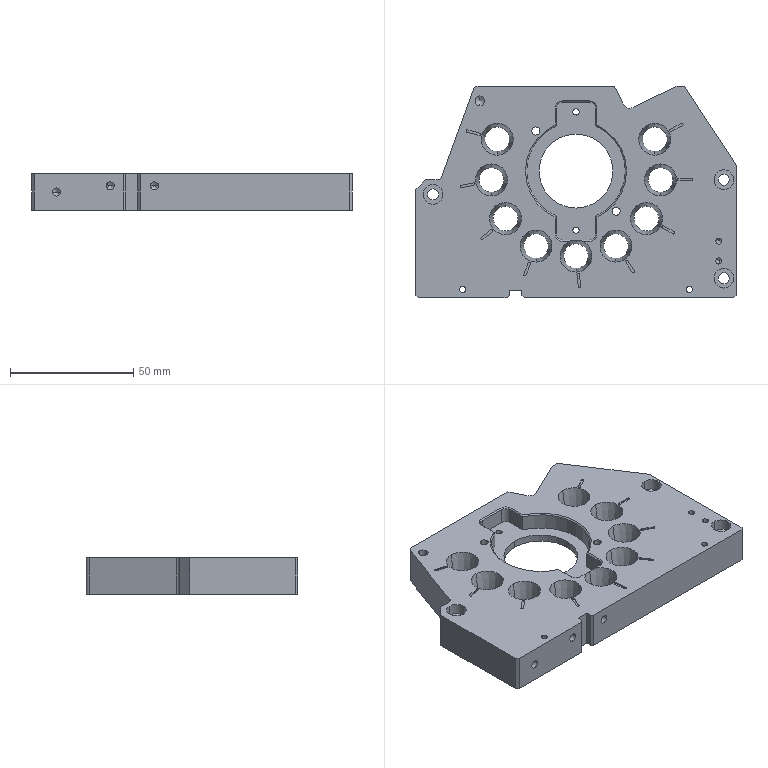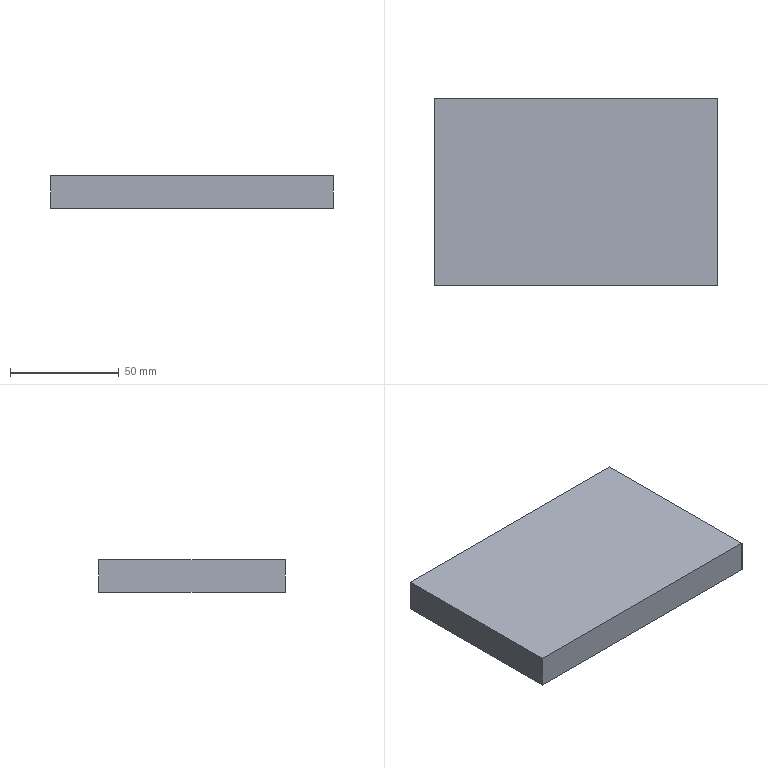CAM job | NX | 3+2 milling, drilling | part box 130 x 86 x 15 mm | stock box 130 x 86 x 15 mm
Tools:
number,name,description,diameter,corner_radius,flute_length,length,flutes
21,ZXZ,Milling Tool-5 Parameters,6.0,0.0,50.0,75.0,2
22,2.5ZT,Drilling Tool,2.5,0.0,35.0,50.0,2
13,3.3ZT,Drilling Tool,3.3,0.0,35.0,50.0,2
24,4.0ZT,Drilling Tool,4.0,0.0,35.0,50.0,2
12,4.5ZT,Drilling Tool,4.5,0.0,35.0,50.0,2
4,D10,Milling Tool-5 Parameters,10.0,0.0,50.0,75.0,2
20,10.ZT,Drilling Tool,10.0,0.0,35.0,50.0,2
17,D4,Milling Tool-5 Parameters,4.0,0.0,50.0,75.0,2
6,D6,Milling Tool-5 Parameters,6.0,0.0,50.0,75.0,2
16,D6JING,Milling Tool-5 Parameters,6.0,0.0,50.0,75.0,2
7,D4R0.5,Milling Tool-5 Parameters,4.0,0.5,50.0,75.0,2
19,D1,Milling Tool-5 Parameters,1.0,0.0,50.0,75.0,2
1,D6A45,Milling Tool-5 Parameters,6.0,0.0,50.0,75.0,2
Operations:
program,operation,operation_type,tool,method,geometry_group,spindle_rpm,surface_speed,feed_per_tooth,feed_cut,feed_plunge,cut_length_mm,path_length_mm,cut_time_min,machine_time_min
1,DRILLING,Operation,ZXZ,METHOD,A,3500.0,65.0,0.0357,250.0,0.0,84.0,690.801,0.336,0.3967
1,DRILLING_COPY_COPY,Operation,2.5ZT,METHOD,A,2000.0,21.0,0.0375,150.0,0.0,103.507,485.801,0.69,0.7283
1,DRILLING_COPY_1,Operation,3.3ZT,METHOD,A,2000.0,21.0,0.0375,150.0,0.0,30.983,171.063,0.2066,0.2206
1,DRILLING_COPY_1_COPY,Operation,4.0ZT,METHOD,A,2000.0,21.0,0.0375,150.0,0.0,9.202,78.403,0.0613,0.0683
1,DRILLING_COPY,Operation,4.5ZT,METHOD,A,2000.0,28.0,0.0375,150.0,0.0,62.556,349.414,0.417,0.4457
1,DRILLING_COPY_COPY_1,Operation,10.ZT,METHOD,A,2000.0,28.0,0.0375,150.0,0.0,202.539,624.758,1.35,1.393
1,ZLEVEL_PROFILE,ZLevelMilling,D10,METHOD,A,3500.0,109.0,0.3143,2200.0,1000.0,9960.656,10284.389,4.731,4.763
1,ADAPTIVE_MILLING,CavityMilling,D10,METHOD,A,7500.0,235.0,0.2,3000.0,1000.0,11162.735,11585.71,5.695,5.738
1,HOLE_MILLING_COPY,CylinderMilling,D6,METHOD,A,5500.0,103.0,0.1364,1500.0,100.0,989.723,1340.176,0.6598,0.6949
1,FLOOR_WALL_1_COPY,VolumeBased25DMillingOperation,D6JING,METHOD,A,7500.0,235.0,0.08,1200.0,1000.0,568.072,639.972,0.4743,0.4815
1,ZLEVEL_PROFILE_2,ZLevelMilling,D6JING,METHOD,A,7500.0,235.0,0.0667,1000.0,100.0,152.755,468.87,0.1528,0.1844
1,ZLEVEL_PROFILE_2_COPY,ZLevelMilling,D6JING,METHOD,A,7500.0,235.0,0.0667,1000.0,100.0,68.474,241.468,0.0685,0.0858
1,ZLEVEL_PROFILE_1,ZLevelMilling,D4,METHOD,A,6500.0,81.0,0.1269,1650.0,100.0,2028.876,3364.187,1.23,1.363
1,ZLEVEL_PROFILE_1_COPY,ZLevelMilling,D4,METHOD,A,6500.0,81.0,0.1269,1650.0,100.0,2070.891,3417.953,1.255,1.39
1,ZLEVEL_PROFILE_1_1,ZLevelMilling,D4R0.5,METHOD,A,7500.0,94.0,0.1667,2500.0,1000.0,22890.897,23935.847,9.168,9.273
1,PLANAR_PROFILE,PlanarMilling,D1,METHOD,A,6500.0,20.0,0.0615,800.0,100.0,4954.5,5607.402,6.193,6.258
1,PLANAR_MILL,PlanarMilling,D6A45,METHOD,A,7500.0,141.0,0.0833,1250.0,100.0,531.11,1965.382,0.4249,0.5683
1,PLANAR_MILL_COPY_1,PlanarMilling,D6A45,METHOD,A,7500.0,141.0,0.0833,1250.0,100.0,96.783,168.783,0.0774,0.0846
1,PLANAR_MILL_COPY,PlanarMilling,D6A45,METHOD,A,7500.0,141.0,0.0833,1250.0,100.0,158.298,217.298,0.1266,0.1325
1,刀补16,ZLevelMilling,D6JING,METHOD,A,7500.0,235.0,0.0667,1000.0,100.0,101.807,250.637,0.1018,0.1167
1,刀补16_COPY,ZLevelMilling,D4,METHOD,A,7500.0,235.0,0.0667,1000.0,100.0,86.152,164.152,0.0862,0.094
2,ADAPTIVE_MILLING_COPY,CavityMilling,D10,METHOD,B,7500.0,235.0,0.2,3000.0,1000.0,11734.765,12049.371,4.22,4.251
2,FLOOR_WALL_1_COPY_COPY,VolumeBased25DMillingOperation,D6JING,METHOD,B,7500.0,235.0,0.08,1200.0,1000.0,702.647,770.547,0.5864,0.5932
2,ZLEVEL_PROFILE_1_COPY_COPY,ZLevelMilling,D4,METHOD,B,6500.0,81.0,0.1269,1650.0,100.0,1560.563,2689.973,0.9458,1.059
2,PLANAR_MILL_COPY_1_COPY,PlanarMilling,D6A45,METHOD,B,7500.0,141.0,0.0833,1250.0,100.0,96.783,164.783,0.0774,0.0842
2,PLANAR_MILL_COPY_1_COPY_COPY,PlanarMilling,D6A45,METHOD,B,7500.0,141.0,0.0833,1250.0,100.0,568.881,1935.207,0.4551,0.5917
3,DRILLING_COPY_2,Operation,ZXZ,METHOD,C,3500.0,65.0,0.0357,250.0,0.0,12.0,152.039,0.048,0.062
3,DRILLING_COPY_1_COPY_1,Operation,3.3ZT,METHOD,C,2000.0,21.0,0.0375,150.0,0.0,37.174,202.388,0.2478,0.2643
3,ZLEVEL_PROFILE_1_COPY_COPY_1,ZLevelMilling,D4,METHOD,C,7500.0,141.0,0.11,1650.0,1000.0,1450.778,1512.678,0.8802,0.8864
3,PLANAR_MILL_COPY_1_COPY_COPY_1,PlanarMilling,D6A45,METHOD,C,7500.0,141.0,0.0833,1250.0,100.0,45.891,166.491,0.0367,0.0488
3,PLANAR_MILL_COPY_1_COPY_COPY_1_COPY,PlanarMilling,D6A45,METHOD,C,7500.0,141.0,0.0833,1250.0,100.0,48.398,264.318,0.0387,0.0603
3,刀补16_1,ZLevelMilling,D4,METHOD,C,7500.0,141.0,0.0667,1000.0,1000.0,57.09,177.171,0.0571,0.0691